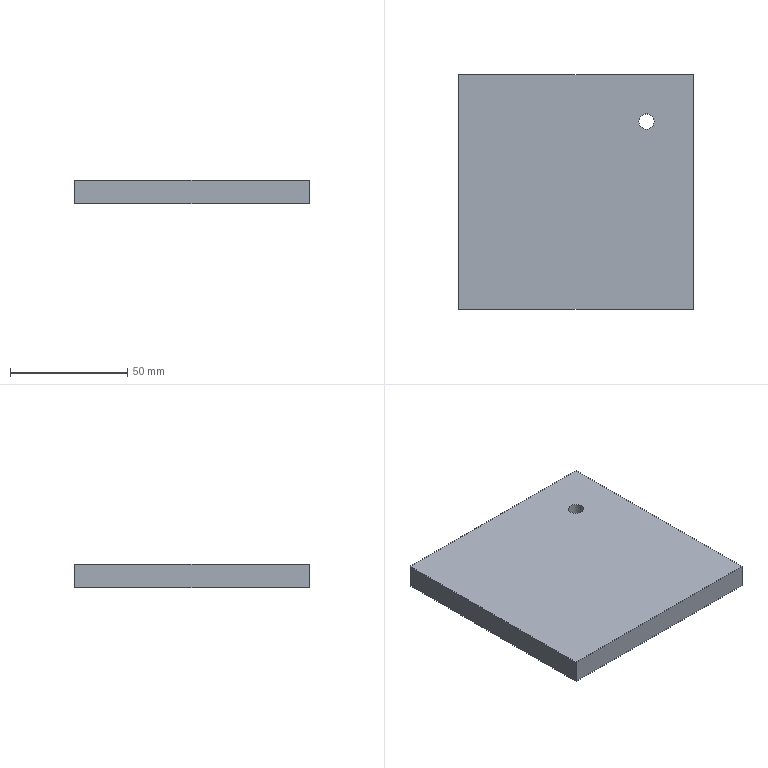Part | STEP file | SynoNew-0304-042 | 1 solid | 7 faces | box 100 x 100 x 10 mm | volume 99668 mm3 | plane 6 | cylinder 1 | commonest cylinder face diameters 6.5 x1
STEP:
#1=CARTESIAN_POINT('',(33.25,30.,10.));
#2=VERTEX_POINT('',#1);
#3=CARTESIAN_POINT('',(26.75,30.,10.));
#4=VERTEX_POINT('',#3);
#5=CARTESIAN_POINT('',(30.,30.,10.));
#6=DIRECTION('',(0.,0.,-1.));
#7=DIRECTION('',(1.,0.,0.));
#8=AXIS2_PLACEMENT_3D('',#5,#6,#7);
#9=CIRCLE('',#8,3.25);
#10=EDGE_CURVE('',#2,#4,#9,.T.);
#11=ORIENTED_EDGE('',*,*,#10,.F.);
#12=CARTESIAN_POINT('',(30.,30.,10.));
#13=DIRECTION('',(0.,0.,-1.));
#14=DIRECTION('',(1.,0.,0.));
#15=AXIS2_PLACEMENT_3D('',#12,#13,#14);
#16=CIRCLE('',#15,3.25);
#17=EDGE_CURVE('',#4,#2,#16,.T.);
#18=ORIENTED_EDGE('',*,*,#17,.F.);
#19=CARTESIAN_POINT('',(26.75,30.,0.));
#20=VERTEX_POINT('',#19);
#21=CARTESIAN_POINT('',(26.75,30.,-131.774));
#22=DIRECTION('',(0.,0.,-1.));
#23=VECTOR('',#22,3.25);
#24=LINE('',#21,#23);
#25=EDGE_CURVE('',#4,#20,#24,.T.);
#26=ORIENTED_EDGE('',*,*,#25,.T.);
#27=CARTESIAN_POINT('',(30.,30.,0.));
#28=DIRECTION('',(0.,0.,1.));
#29=DIRECTION('',(1.,0.,0.));
#30=AXIS2_PLACEMENT_3D('',#27,#28,#29);
#31=CIRCLE('',#30,3.25);
#32=EDGE_CURVE('',#20,#20,#31,.T.);
#33=ORIENTED_EDGE('',*,*,#32,.F.);
#34=ORIENTED_EDGE('',*,*,#25,.F.);
#35=EDGE_LOOP('',(#11,#18,#26,#33,#34));
#36=FACE_OUTER_BOUND('',#35,.T.);
#37=CARTESIAN_POINT('',(30.,30.,-131.774));
#38=DIRECTION('',(0.,0.,1.));
#39=DIRECTION('',(1.,0.,0.));
#40=AXIS2_PLACEMENT_3D('',#37,#38,#39);
#41=CYLINDRICAL_SURFACE('',#40,3.25);
#42=ADVANCED_FACE('',(#36),#41,.F.);
#43=CARTESIAN_POINT('',(-50.,-50.,0.));
#44=VERTEX_POINT('',#43);
#45=CARTESIAN_POINT('',(50.,-50.,0.));
#46=VERTEX_POINT('',#45);
#47=CARTESIAN_POINT('',(-50.,-50.,0.));
#48=DIRECTION('',(1.,0.,0.));
#49=VECTOR('',#48,10.);
#50=LINE('',#47,#49);
#51=EDGE_CURVE('',#44,#46,#50,.T.);
#52=ORIENTED_EDGE('',*,*,#51,.T.);
#53=CARTESIAN_POINT('',(50.,-50.,10.));
#54=VERTEX_POINT('',#53);
#55=CARTESIAN_POINT('',(50.,-50.,0.));
#56=DIRECTION('',(0.,0.,1.));
#57=VECTOR('',#56,10.);
#58=LINE('',#55,#57);
#59=EDGE_CURVE('',#46,#54,#58,.T.);
#60=ORIENTED_EDGE('',*,*,#59,.T.);
#61=CARTESIAN_POINT('',(-50.,-50.,10.));
#62=VERTEX_POINT('',#61);
#63=CARTESIAN_POINT('',(-50.,-50.,10.));
#64=DIRECTION('',(1.,0.,0.));
#65=VECTOR('',#64,10.);
#66=LINE('',#63,#65);
#67=EDGE_CURVE('',#62,#54,#66,.T.);
#68=ORIENTED_EDGE('',*,*,#67,.F.);
#69=CARTESIAN_POINT('',(-50.,-50.,0.));
#70=DIRECTION('',(0.,0.,1.));
#71=VECTOR('',#70,10.);
#72=LINE('',#69,#71);
#73=EDGE_CURVE('',#44,#62,#72,.T.);
#74=ORIENTED_EDGE('',*,*,#73,.F.);
#75=EDGE_LOOP('',(#52,#60,#68,#74));
#76=FACE_OUTER_BOUND('',#75,.T.);
#77=CARTESIAN_POINT('',(-50.,-50.,0.));
#78=DIRECTION('',(0.,-1.,0.));
#79=DIRECTION('',(1.,0.,0.));
#80=AXIS2_PLACEMENT_3D('',#77,#78,#79);
#81=PLANE('',#80);
#82=ADVANCED_FACE('',(#76),#81,.T.);
#83=CARTESIAN_POINT('',(-50.,50.,0.));
#84=VERTEX_POINT('',#83);
#85=CARTESIAN_POINT('',(-50.,50.,0.));
#86=DIRECTION('',(0.,-1.,0.));
#87=VECTOR('',#86,10.);
#88=LINE('',#85,#87);
#89=EDGE_CURVE('',#84,#44,#88,.T.);
#90=ORIENTED_EDGE('',*,*,#89,.T.);
#91=ORIENTED_EDGE('',*,*,#73,.T.);
#92=CARTESIAN_POINT('',(-50.,50.,10.));
#93=VERTEX_POINT('',#92);
#94=CARTESIAN_POINT('',(-50.,50.,10.));
#95=DIRECTION('',(0.,-1.,0.));
#96=VECTOR('',#95,10.);
#97=LINE('',#94,#96);
#98=EDGE_CURVE('',#93,#62,#97,.T.);
#99=ORIENTED_EDGE('',*,*,#98,.F.);
#100=CARTESIAN_POINT('',(-50.,50.,0.));
#101=DIRECTION('',(0.,0.,1.));
#102=VECTOR('',#101,10.);
#103=LINE('',#100,#102);
#104=EDGE_CURVE('',#84,#93,#103,.T.);
#105=ORIENTED_EDGE('',*,*,#104,.F.);
#106=EDGE_LOOP('',(#90,#91,#99,#105));
#107=FACE_OUTER_BOUND('',#106,.T.);
#108=CARTESIAN_POINT('',(-50.,50.,0.));
#109=DIRECTION('',(-1.,0.,0.));
#110=DIRECTION('',(0.,-1.,0.));
#111=AXIS2_PLACEMENT_3D('',#108,#109,#110);
#112=PLANE('',#111);
#113=ADVANCED_FACE('',(#107),#112,.T.);
#114=CARTESIAN_POINT('',(50.,50.,0.));
#115=VERTEX_POINT('',#114);
#116=CARTESIAN_POINT('',(50.,50.,0.));
#117=DIRECTION('',(-1.,0.,0.));
#118=VECTOR('',#117,10.);
#119=LINE('',#116,#118);
#120=EDGE_CURVE('',#115,#84,#119,.T.);
#121=ORIENTED_EDGE('',*,*,#120,.T.);
#122=ORIENTED_EDGE('',*,*,#104,.T.);
#123=CARTESIAN_POINT('',(50.,50.,10.));
#124=VERTEX_POINT('',#123);
#125=CARTESIAN_POINT('',(50.,50.,10.));
#126=DIRECTION('',(-1.,0.,0.));
#127=VECTOR('',#126,10.);
#128=LINE('',#125,#127);
#129=EDGE_CURVE('',#124,#93,#128,.T.);
#130=ORIENTED_EDGE('',*,*,#129,.F.);
#131=CARTESIAN_POINT('',(50.,50.,0.));
#132=DIRECTION('',(0.,0.,1.));
#133=VECTOR('',#132,10.);
#134=LINE('',#131,#133);
#135=EDGE_CURVE('',#115,#124,#134,.T.);
#136=ORIENTED_EDGE('',*,*,#135,.F.);
#137=EDGE_LOOP('',(#121,#122,#130,#136));
#138=FACE_OUTER_BOUND('',#137,.T.);
#139=CARTESIAN_POINT('',(50.,50.,0.));
#140=DIRECTION('',(0.,1.,0.));
#141=DIRECTION('',(-1.,0.,0.));
#142=AXIS2_PLACEMENT_3D('',#139,#140,#141);
#143=PLANE('',#142);
#144=ADVANCED_FACE('',(#138),#143,.T.);
#145=CARTESIAN_POINT('',(50.,-50.,0.));
#146=DIRECTION('',(0.,1.,0.));
#147=VECTOR('',#146,10.);
#148=LINE('',#145,#147);
#149=EDGE_CURVE('',#46,#115,#148,.T.);
#150=ORIENTED_EDGE('',*,*,#149,.T.);
#151=ORIENTED_EDGE('',*,*,#135,.T.);
#152=CARTESIAN_POINT('',(50.,-50.,10.));
#153=DIRECTION('',(0.,1.,0.));
#154=VECTOR('',#153,10.);
#155=LINE('',#152,#154);
#156=EDGE_CURVE('',#54,#124,#155,.T.);
#157=ORIENTED_EDGE('',*,*,#156,.F.);
#158=ORIENTED_EDGE('',*,*,#59,.F.);
#159=EDGE_LOOP('',(#150,#151,#157,#158));
#160=FACE_OUTER_BOUND('',#159,.T.);
#161=CARTESIAN_POINT('',(50.,-50.,0.));
#162=DIRECTION('',(1.,0.,0.));
#163=DIRECTION('',(0.,1.,0.));
#164=AXIS2_PLACEMENT_3D('',#161,#162,#163);
#165=PLANE('',#164);
#166=ADVANCED_FACE('',(#160),#165,.T.);
#167=ORIENTED_EDGE('',*,*,#156,.T.);
#168=ORIENTED_EDGE('',*,*,#129,.T.);
#169=ORIENTED_EDGE('',*,*,#98,.T.);
#170=ORIENTED_EDGE('',*,*,#67,.T.);
#171=EDGE_LOOP('',(#167,#168,#169,#170));
#172=FACE_OUTER_BOUND('',#171,.T.);
#173=ORIENTED_EDGE('',*,*,#10,.T.);
#174=ORIENTED_EDGE('',*,*,#17,.T.);
#175=EDGE_LOOP('',(#173,#174));
#176=FACE_BOUND('',#175,.T.);
#177=CARTESIAN_POINT('',(0.,0.,10.));
#178=DIRECTION('',(0.,0.,1.));
#179=DIRECTION('',(1.,0.,0.));
#180=AXIS2_PLACEMENT_3D('',#177,#178,#179);
#181=PLANE('',#180);
#182=ADVANCED_FACE('',(#172,#176),#181,.T.);
#183=ORIENTED_EDGE('',*,*,#149,.F.);
#184=ORIENTED_EDGE('',*,*,#51,.F.);
#185=ORIENTED_EDGE('',*,*,#89,.F.);
#186=ORIENTED_EDGE('',*,*,#120,.F.);
#187=EDGE_LOOP('',(#183,#184,#185,#186));
#188=FACE_OUTER_BOUND('',#187,.T.);
#189=ORIENTED_EDGE('',*,*,#32,.T.);
#190=EDGE_LOOP('',(#189));
#191=FACE_BOUND('',#190,.T.);
#192=CARTESIAN_POINT('',(0.,0.,0.));
#193=DIRECTION('',(0.,0.,1.));
#194=DIRECTION('',(1.,0.,0.));
#195=AXIS2_PLACEMENT_3D('',#192,#193,#194);
#196=PLANE('',#195);
#197=ADVANCED_FACE('',(#188,#191),#196,.F.);
#198=CLOSED_SHELL('',(#42,#82,#113,#144,#166,#182,#197));
#199=MANIFOLD_SOLID_BREP('',#198);
#200=(LENGTH_UNIT()NAMED_UNIT(*)SI_UNIT(.MILLI.,.METRE.));
#201=UNCERTAINTY_MEASURE_WITH_UNIT(LENGTH_MEASURE(0.01),#200,'','');
#202=(NAMED_UNIT(*)PLANE_ANGLE_UNIT()SI_UNIT($,.RADIAN.));
#203=(NAMED_UNIT(*)SI_UNIT($,.STERADIAN.)SOLID_ANGLE_UNIT());
#204=(GEOMETRIC_REPRESENTATION_CONTEXT(3)GLOBAL_UNCERTAINTY_ASSIGNED_CONTEXT((#201))GLOBAL_UNIT_ASSIGNED_CONTEXT((#200,#202,#203))REPRESENTATION_CONTEXT('',''));
#205=ADVANCED_BREP_SHAPE_REPRESENTATION('',(#199),#204);